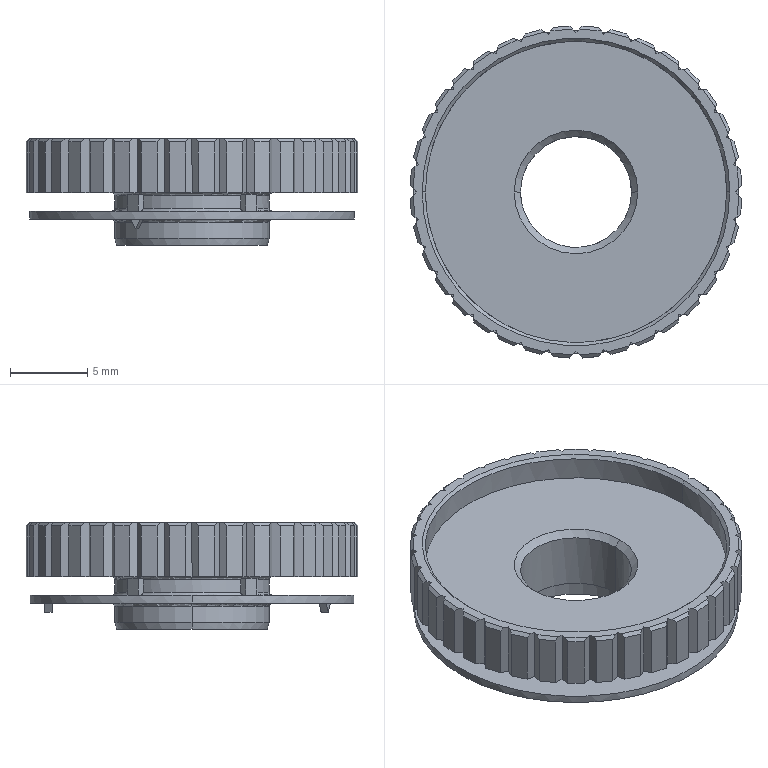Part | SolidWorks | features BaseBody 1 | 1 solid | 203 faces | box 21.485 x 21.485 x 6.9 mm | volume 915.19 mm3 | plane 103 | cylinder 50 | cone 42 | torus 8 | commonest cylinder face diameters 21.5 x36 10 x6 7.188 x2 8.2 x2 19.5 x2 21 x2